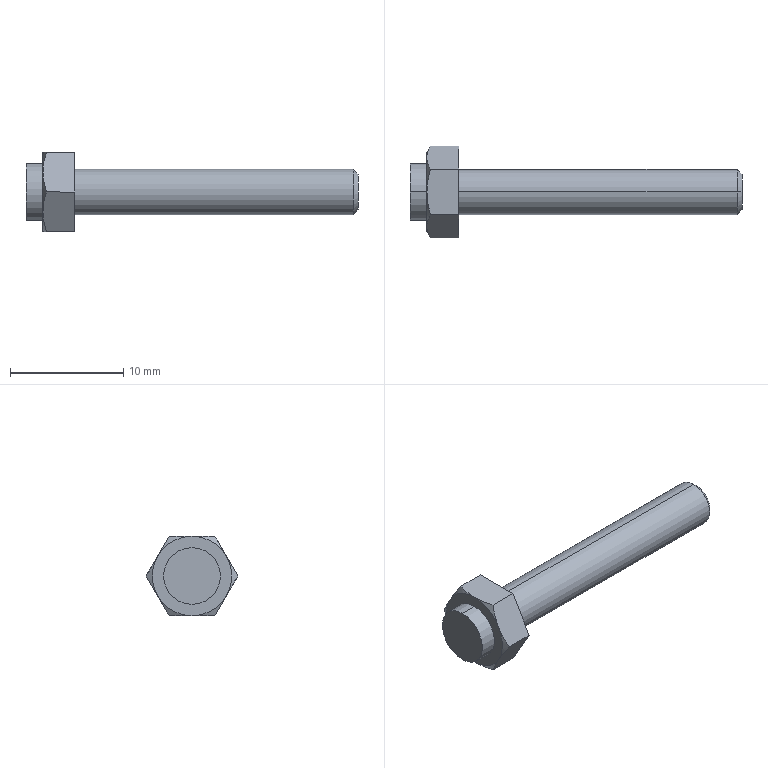Part | STEP file | 0246_Z_002_PUST4-25_1 | 1 solid | 22 faces | box 29.3 x 8.083 x 7 mm | volume 460.98 mm3 | plane 10 | cone 8 | cylinder 4 | commonest cylinder face diameters 4 x2 5 x2